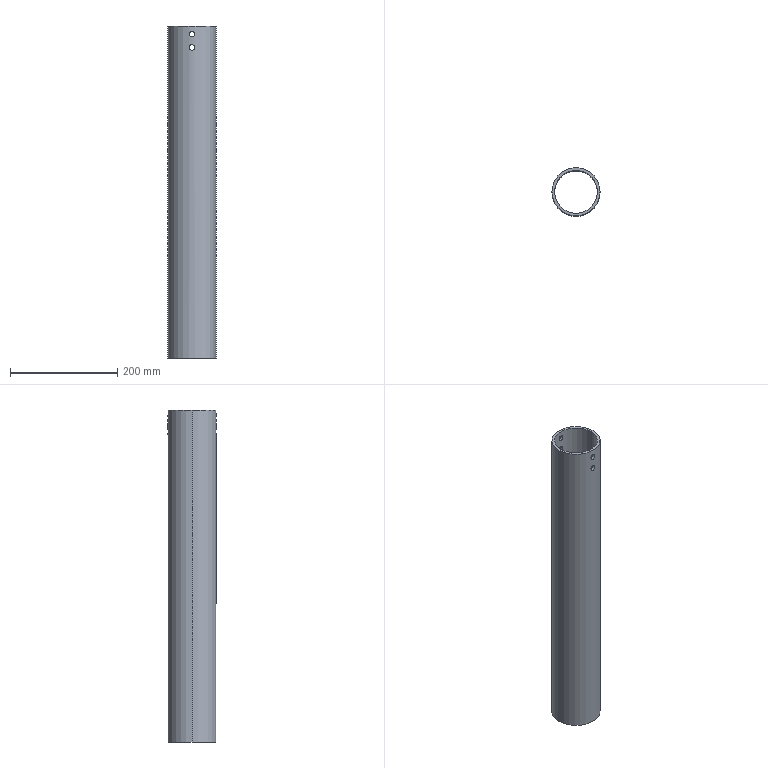Part | SolidWorks | features ICE 3, Cut 1, Extrusion 1 | 1 solid | 14 faces | box 90 x 90 x 620 mm | volume 826172 mm3 | cylinder 12 | plane 2 | commonest cylinder face diameters 10.2 x8 80 x2 90 x2
STEP:
#1=CARTESIAN_POINT('',(0.,-45.,599.9));
#2=VERTEX_POINT('',#1);
#3=CARTESIAN_POINT('',(0.,-45.,610.1));
#4=VERTEX_POINT('',#3);
#5=CARTESIAN_POINT('',(0.,-45.,599.9));
#6=CARTESIAN_POINT('',(-0.3329,-45.,599.9));
#7=CARTESIAN_POINT('',(-0.664,-44.996,599.932));
#8=CARTESIAN_POINT('',(-1.322,-44.982,600.063));
#9=CARTESIAN_POINT('',(-1.644,-44.971,600.161));
#10=CARTESIAN_POINT('',(-2.258,-44.944,600.415));
#11=CARTESIAN_POINT('',(-2.555,-44.928,600.573));
#12=CARTESIAN_POINT('',(-3.112,-44.893,600.946));
#13=CARTESIAN_POINT('',(-3.369,-44.874,601.156));
#14=CARTESIAN_POINT('',(-3.839,-44.837,601.626));
#15=CARTESIAN_POINT('',(-4.054,-44.817,601.888));
#16=CARTESIAN_POINT('',(-4.425,-44.782,602.442));
#17=CARTESIAN_POINT('',(-4.581,-44.766,602.735));
#18=CARTESIAN_POINT('',(-4.774,-44.746,603.198));
#19=CARTESIAN_POINT('',(-4.831,-44.74,603.357));
#20=CARTESIAN_POINT('',(-4.928,-44.729,603.677));
#21=CARTESIAN_POINT('',(-4.969,-44.725,603.839));
#22=CARTESIAN_POINT('',(-5.066,-44.714,604.328));
#23=CARTESIAN_POINT('',(-5.1,-44.71,604.659));
#24=CARTESIAN_POINT('',(-5.1,-44.71,605.333));
#25=CARTESIAN_POINT('',(-5.067,-44.714,605.665));
#26=CARTESIAN_POINT('',(-4.97,-44.725,606.154));
#27=CARTESIAN_POINT('',(-4.93,-44.729,606.316));
#28=CARTESIAN_POINT('',(-4.833,-44.74,606.636));
#29=CARTESIAN_POINT('',(-4.776,-44.746,606.796));
#30=CARTESIAN_POINT('',(-4.585,-44.766,607.259));
#31=CARTESIAN_POINT('',(-4.428,-44.782,607.552));
#32=CARTESIAN_POINT('',(-4.059,-44.817,608.106));
#33=CARTESIAN_POINT('',(-3.844,-44.836,608.369));
#34=CARTESIAN_POINT('',(-3.374,-44.874,608.839));
#35=CARTESIAN_POINT('',(-3.118,-44.893,609.05));
#36=CARTESIAN_POINT('',(-2.561,-44.928,609.423));
#37=CARTESIAN_POINT('',(-2.264,-44.944,609.582));
#38=CARTESIAN_POINT('',(-1.651,-44.971,609.837));
#39=CARTESIAN_POINT('',(-1.33,-44.982,609.935));
#40=CARTESIAN_POINT('',(-0.6706,-44.996,610.067));
#41=CARTESIAN_POINT('',(-0.3372,-45.,610.1));
#42=CARTESIAN_POINT('',(0.,-45.,610.1));
#43=B_SPLINE_CURVE_WITH_KNOTS('',3,(#5,#6,#7,#8,#9,#10,#11,#12,#13,#14,#15,#16,#17,#18,#19,#20,#21,#22,#23,#24,#25,#26,#27,#28,#29,#30,#31,#32,#33,#34,#35,#36,#37,#38,#39,#40,#41,#42),.UNSPECIFIED.,.F.,.F.,(4,2,2,2,2,2,2,2,2,2,2,2,2,2,2,2,2,2,4),(0.01596,0.01695,0.01795,0.01895,0.01995,0.02094,0.02194,0.02244,0.02294,0.02393,0.02493,0.02543,0.02593,0.02693,0.02792,0.02892,0.02992,0.03091,0.03191),.UNSPECIFIED.);
#44=EDGE_CURVE('',#2,#4,#43,.T.);
#45=ORIENTED_EDGE('',*,*,#44,.F.);
#46=CARTESIAN_POINT('',(0.,-40.,599.9));
#47=VERTEX_POINT('',#46);
#48=CARTESIAN_POINT('',(0.,-91.,599.9));
#49=DIRECTION('',(0.,1.,0.));
#50=VECTOR('',#49,1000.);
#51=LINE('',#48,#50);
#52=EDGE_CURVE('',#2,#47,#51,.T.);
#53=ORIENTED_EDGE('',*,*,#52,.T.);
#54=CARTESIAN_POINT('',(0.,-40.,610.1));
#55=VERTEX_POINT('',#54);
#56=CARTESIAN_POINT('',(0.,-40.,599.9));
#57=CARTESIAN_POINT('',(-0.3329,-40.,599.9));
#58=CARTESIAN_POINT('',(-0.6641,-39.996,599.932));
#59=CARTESIAN_POINT('',(-1.323,-39.979,600.063));
#60=CARTESIAN_POINT('',(-1.644,-39.967,600.161));
#61=CARTESIAN_POINT('',(-2.258,-39.937,600.415));
#62=CARTESIAN_POINT('',(-2.555,-39.919,600.573));
#63=CARTESIAN_POINT('',(-3.112,-39.88,600.946));
#64=CARTESIAN_POINT('',(-3.369,-39.859,601.156));
#65=CARTESIAN_POINT('',(-3.839,-39.816,601.626));
#66=CARTESIAN_POINT('',(-4.054,-39.794,601.888));
#67=CARTESIAN_POINT('',(-4.425,-39.755,602.442));
#68=CARTESIAN_POINT('',(-4.581,-39.737,602.734));
#69=CARTESIAN_POINT('',(-4.774,-39.714,603.197));
#70=CARTESIAN_POINT('',(-4.831,-39.707,603.357));
#71=CARTESIAN_POINT('',(-4.928,-39.695,603.677));
#72=CARTESIAN_POINT('',(-4.969,-39.69,603.839));
#73=CARTESIAN_POINT('',(-5.066,-39.678,604.328));
#74=CARTESIAN_POINT('',(-5.1,-39.674,604.659));
#75=CARTESIAN_POINT('',(-5.1,-39.674,605.334));
#76=CARTESIAN_POINT('',(-5.067,-39.678,605.665));
#77=CARTESIAN_POINT('',(-4.97,-39.69,606.154));
#78=CARTESIAN_POINT('',(-4.93,-39.695,606.316));
#79=CARTESIAN_POINT('',(-4.833,-39.707,606.637));
#80=CARTESIAN_POINT('',(-4.776,-39.714,606.796));
#81=CARTESIAN_POINT('',(-4.585,-39.737,607.259));
#82=CARTESIAN_POINT('',(-4.428,-39.755,607.552));
#83=CARTESIAN_POINT('',(-4.058,-39.794,608.107));
#84=CARTESIAN_POINT('',(-3.843,-39.816,608.369));
#85=CARTESIAN_POINT('',(-3.374,-39.858,608.839));
#86=CARTESIAN_POINT('',(-3.118,-39.879,609.05));
#87=CARTESIAN_POINT('',(-2.56,-39.919,609.423));
#88=CARTESIAN_POINT('',(-2.264,-39.937,609.582));
#89=CARTESIAN_POINT('',(-1.651,-39.967,609.837));
#90=CARTESIAN_POINT('',(-1.33,-39.979,609.935));
#91=CARTESIAN_POINT('',(-0.6707,-39.996,610.067));
#92=CARTESIAN_POINT('',(-0.3373,-40.,610.1));
#93=CARTESIAN_POINT('',(0.,-40.,610.1));
#94=B_SPLINE_CURVE_WITH_KNOTS('',3,(#56,#57,#58,#59,#60,#61,#62,#63,#64,#65,#66,#67,#68,#69,#70,#71,#72,#73,#74,#75,#76,#77,#78,#79,#80,#81,#82,#83,#84,#85,#86,#87,#88,#89,#90,#91,#92,#93),.UNSPECIFIED.,.F.,.F.,(4,2,2,2,2,2,2,2,2,2,2,2,2,2,2,2,2,2,4),(0.01596,0.01696,0.01796,0.01895,0.01995,0.02095,0.02195,0.02244,0.02294,0.02394,0.02494,0.02544,0.02593,0.02693,0.02793,0.02893,0.02992,0.03092,0.03192),.UNSPECIFIED.);
#95=EDGE_CURVE('',#47,#55,#94,.T.);
#96=ORIENTED_EDGE('',*,*,#95,.T.);
#97=CARTESIAN_POINT('',(0.,-91.,610.1));
#98=DIRECTION('',(0.,1.,0.));
#99=VECTOR('',#98,1000.);
#100=LINE('',#97,#99);
#101=EDGE_CURVE('',#4,#55,#100,.T.);
#102=ORIENTED_EDGE('',*,*,#101,.F.);
#103=EDGE_LOOP('',(#45,#53,#96,#102));
#104=FACE_OUTER_BOUND('',#103,.T.);
#105=CARTESIAN_POINT('',(0.,-91.,605.));
#106=DIRECTION('',(0.,1.,0.));
#107=DIRECTION('',(0.,0.,1.));
#108=AXIS2_PLACEMENT_3D('',#105,#106,#107);
#109=CYLINDRICAL_SURFACE('',#108,5.1);
#110=ADVANCED_FACE('',(#104),#109,.F.);
#111=CARTESIAN_POINT('',(0.,40.,610.1));
#112=VERTEX_POINT('',#111);
#113=CARTESIAN_POINT('',(0.,40.,599.9));
#114=VERTEX_POINT('',#113);
#115=CARTESIAN_POINT('',(0.,40.,610.1));
#116=CARTESIAN_POINT('',(-0.3373,40.,610.1));
#117=CARTESIAN_POINT('',(-0.669,39.996,610.067));
#118=CARTESIAN_POINT('',(-1.158,39.984,609.97));
#119=CARTESIAN_POINT('',(-1.32,39.979,609.929));
#120=CARTESIAN_POINT('',(-1.641,39.967,609.832));
#121=CARTESIAN_POINT('',(-1.8,39.96,609.775));
#122=CARTESIAN_POINT('',(-2.263,39.937,609.583));
#123=CARTESIAN_POINT('',(-2.556,39.919,609.426));
#124=CARTESIAN_POINT('',(-3.11,39.88,609.056));
#125=CARTESIAN_POINT('',(-3.372,39.858,608.841));
#126=CARTESIAN_POINT('',(-3.842,39.816,608.37));
#127=CARTESIAN_POINT('',(-4.053,39.795,608.114));
#128=CARTESIAN_POINT('',(-4.426,39.755,607.556));
#129=CARTESIAN_POINT('',(-4.584,39.737,607.26));
#130=CARTESIAN_POINT('',(-4.838,39.707,606.646));
#131=CARTESIAN_POINT('',(-4.936,39.694,606.325));
#132=CARTESIAN_POINT('',(-5.067,39.678,605.666));
#133=CARTESIAN_POINT('',(-5.1,39.674,605.335));
#134=CARTESIAN_POINT('',(-5.1,39.674,604.669));
#135=CARTESIAN_POINT('',(-5.067,39.678,604.331));
#136=CARTESIAN_POINT('',(-4.936,39.694,603.676));
#137=CARTESIAN_POINT('',(-4.84,39.706,603.358));
#138=CARTESIAN_POINT('',(-4.648,39.729,602.895));
#139=CARTESIAN_POINT('',(-4.576,39.737,602.742));
#140=CARTESIAN_POINT('',(-4.418,39.755,602.447));
#141=CARTESIAN_POINT('',(-4.332,39.765,602.304));
#142=CARTESIAN_POINT('',(-4.055,39.794,601.89));
#143=CARTESIAN_POINT('',(-3.844,39.816,601.632));
#144=CARTESIAN_POINT('',(-3.369,39.859,601.156));
#145=CARTESIAN_POINT('',(-3.111,39.88,600.945));
#146=CARTESIAN_POINT('',(-2.697,39.909,600.669));
#147=CARTESIAN_POINT('',(-2.555,39.919,600.583));
#148=CARTESIAN_POINT('',(-2.259,39.936,600.425));
#149=CARTESIAN_POINT('',(-2.107,39.945,600.352));
#150=CARTESIAN_POINT('',(-1.644,39.967,600.161));
#151=CARTESIAN_POINT('',(-1.326,39.979,600.064));
#152=CARTESIAN_POINT('',(-0.6713,39.996,599.933));
#153=CARTESIAN_POINT('',(-0.333,40.,599.9));
#154=CARTESIAN_POINT('',(0.,40.,599.9));
#155=B_SPLINE_CURVE_WITH_KNOTS('',3,(#115,#116,#117,#118,#119,#120,#121,#122,#123,#124,#125,#126,#127,#128,#129,#130,#131,#132,#133,#134,#135,#136,#137,#138,#139,#140,#141,#142,#143,#144,#145,#146,#147,#148,#149,#150,#151,#152,#153,#154),.UNSPECIFIED.,.F.,.F.,(4,2,2,2,2,2,2,2,2,2,2,2,2,2,2,2,2,2,2,4),(0.,0.0009976,0.001496,0.001995,0.002993,0.00399,0.004988,0.005985,0.006983,0.007981,0.008978,0.009976,0.01047,0.01097,0.01197,0.01297,0.01347,0.01397,0.01496,0.01596),.UNSPECIFIED.);
#156=EDGE_CURVE('',#112,#114,#155,.T.);
#157=ORIENTED_EDGE('',*,*,#156,.T.);
#158=CARTESIAN_POINT('',(0.,45.,599.9));
#159=VERTEX_POINT('',#158);
#160=CARTESIAN_POINT('',(0.,-91.,599.9));
#161=DIRECTION('',(0.,1.,0.));
#162=VECTOR('',#161,1000.);
#163=LINE('',#160,#162);
#164=EDGE_CURVE('',#114,#159,#163,.T.);
#165=ORIENTED_EDGE('',*,*,#164,.T.);
#166=CARTESIAN_POINT('',(0.,45.,610.1));
#167=VERTEX_POINT('',#166);
#168=CARTESIAN_POINT('',(0.,45.,610.1));
#169=CARTESIAN_POINT('',(-0.3373,45.,610.1));
#170=CARTESIAN_POINT('',(-0.6688,44.996,610.067));
#171=CARTESIAN_POINT('',(-1.158,44.985,609.97));
#172=CARTESIAN_POINT('',(-1.32,44.981,609.929));
#173=CARTESIAN_POINT('',(-1.64,44.97,609.832));
#174=CARTESIAN_POINT('',(-1.8,44.964,609.775));
#175=CARTESIAN_POINT('',(-2.263,44.944,609.583));
#176=CARTESIAN_POINT('',(-2.556,44.928,609.426));
#177=CARTESIAN_POINT('',(-3.11,44.893,609.056));
#178=CARTESIAN_POINT('',(-3.372,44.874,608.841));
#179=CARTESIAN_POINT('',(-3.842,44.836,608.37));
#180=CARTESIAN_POINT('',(-4.053,44.818,608.114));
#181=CARTESIAN_POINT('',(-4.426,44.782,607.556));
#182=CARTESIAN_POINT('',(-4.584,44.766,607.26));
#183=CARTESIAN_POINT('',(-4.838,44.739,606.646));
#184=CARTESIAN_POINT('',(-4.936,44.728,606.324));
#185=CARTESIAN_POINT('',(-5.067,44.714,605.666));
#186=CARTESIAN_POINT('',(-5.1,44.71,605.335));
#187=CARTESIAN_POINT('',(-5.1,44.71,604.669));
#188=CARTESIAN_POINT('',(-5.067,44.714,604.331));
#189=CARTESIAN_POINT('',(-4.937,44.728,603.676));
#190=CARTESIAN_POINT('',(-4.84,44.739,603.358));
#191=CARTESIAN_POINT('',(-4.648,44.759,602.895));
#192=CARTESIAN_POINT('',(-4.576,44.767,602.742));
#193=CARTESIAN_POINT('',(-4.418,44.783,602.447));
#194=CARTESIAN_POINT('',(-4.332,44.791,602.304));
#195=CARTESIAN_POINT('',(-4.056,44.817,601.89));
#196=CARTESIAN_POINT('',(-3.845,44.836,601.632));
#197=CARTESIAN_POINT('',(-3.369,44.874,601.156));
#198=CARTESIAN_POINT('',(-3.111,44.893,600.945));
#199=CARTESIAN_POINT('',(-2.697,44.919,600.668));
#200=CARTESIAN_POINT('',(-2.554,44.928,600.583));
#201=CARTESIAN_POINT('',(-2.259,44.943,600.425));
#202=CARTESIAN_POINT('',(-2.106,44.951,600.352));
#203=CARTESIAN_POINT('',(-1.643,44.971,600.16));
#204=CARTESIAN_POINT('',(-1.325,44.982,600.064));
#205=CARTESIAN_POINT('',(-0.6712,44.996,599.933));
#206=CARTESIAN_POINT('',(-0.333,45.,599.9));
#207=CARTESIAN_POINT('',(0.,45.,599.9));
#208=B_SPLINE_CURVE_WITH_KNOTS('',3,(#168,#169,#170,#171,#172,#173,#174,#175,#176,#177,#178,#179,#180,#181,#182,#183,#184,#185,#186,#187,#188,#189,#190,#191,#192,#193,#194,#195,#196,#197,#198,#199,#200,#201,#202,#203,#204,#205,#206,#207),.UNSPECIFIED.,.F.,.F.,(4,2,2,2,2,2,2,2,2,2,2,2,2,2,2,2,2,2,2,4),(0.,0.0009974,0.001496,0.001995,0.002992,0.003989,0.004987,0.005984,0.006982,0.007979,0.008976,0.009974,0.01047,0.01097,0.01197,0.01297,0.01346,0.01396,0.01496,0.01596),.UNSPECIFIED.);
#209=EDGE_CURVE('',#167,#159,#208,.T.);
#210=ORIENTED_EDGE('',*,*,#209,.F.);
#211=CARTESIAN_POINT('',(0.,-91.,610.1));
#212=DIRECTION('',(0.,1.,0.));
#213=VECTOR('',#212,1000.);
#214=LINE('',#211,#213);
#215=EDGE_CURVE('',#112,#167,#214,.T.);
#216=ORIENTED_EDGE('',*,*,#215,.F.);
#217=EDGE_LOOP('',(#157,#165,#210,#216));
#218=FACE_OUTER_BOUND('',#217,.T.);
#219=CARTESIAN_POINT('',(0.,-91.,605.));
#220=DIRECTION('',(0.,1.,0.));
#221=DIRECTION('',(0.,0.,1.));
#222=AXIS2_PLACEMENT_3D('',#219,#220,#221);
#223=CYLINDRICAL_SURFACE('',#222,5.1);
#224=ADVANCED_FACE('',(#218),#223,.F.);
#225=CARTESIAN_POINT('',(0.,-45.,574.9));
#226=VERTEX_POINT('',#225);
#227=CARTESIAN_POINT('',(0.,-45.,585.1));
#228=VERTEX_POINT('',#227);
#229=CARTESIAN_POINT('',(0.,-45.,574.9));
#230=CARTESIAN_POINT('',(-0.3329,-45.,574.9));
#231=CARTESIAN_POINT('',(-0.664,-44.996,574.932));
#232=CARTESIAN_POINT('',(-1.322,-44.982,575.063));
#233=CARTESIAN_POINT('',(-1.644,-44.971,575.161));
#234=CARTESIAN_POINT('',(-2.258,-44.944,575.415));
#235=CARTESIAN_POINT('',(-2.555,-44.928,575.573));
#236=CARTESIAN_POINT('',(-3.112,-44.893,575.946));
#237=CARTESIAN_POINT('',(-3.369,-44.874,576.156));
#238=CARTESIAN_POINT('',(-3.839,-44.837,576.626));
#239=CARTESIAN_POINT('',(-4.054,-44.817,576.888));
#240=CARTESIAN_POINT('',(-4.425,-44.782,577.442));
#241=CARTESIAN_POINT('',(-4.581,-44.766,577.735));
#242=CARTESIAN_POINT('',(-4.774,-44.746,578.198));
#243=CARTESIAN_POINT('',(-4.831,-44.74,578.357));
#244=CARTESIAN_POINT('',(-4.928,-44.729,578.677));
#245=CARTESIAN_POINT('',(-4.969,-44.725,578.839));
#246=CARTESIAN_POINT('',(-5.066,-44.714,579.328));
#247=CARTESIAN_POINT('',(-5.1,-44.71,579.659));
#248=CARTESIAN_POINT('',(-5.1,-44.71,580.333));
#249=CARTESIAN_POINT('',(-5.067,-44.714,580.665));
#250=CARTESIAN_POINT('',(-4.97,-44.725,581.154));
#251=CARTESIAN_POINT('',(-4.93,-44.729,581.316));
#252=CARTESIAN_POINT('',(-4.833,-44.74,581.636));
#253=CARTESIAN_POINT('',(-4.776,-44.746,581.796));
#254=CARTESIAN_POINT('',(-4.585,-44.766,582.259));
#255=CARTESIAN_POINT('',(-4.428,-44.782,582.552));
#256=CARTESIAN_POINT('',(-4.059,-44.817,583.106));
#257=CARTESIAN_POINT('',(-3.844,-44.836,583.369));
#258=CARTESIAN_POINT('',(-3.374,-44.874,583.839));
#259=CARTESIAN_POINT('',(-3.118,-44.893,584.05));
#260=CARTESIAN_POINT('',(-2.561,-44.928,584.423));
#261=CARTESIAN_POINT('',(-2.264,-44.944,584.582));
#262=CARTESIAN_POINT('',(-1.651,-44.971,584.837));
#263=CARTESIAN_POINT('',(-1.33,-44.982,584.935));
#264=CARTESIAN_POINT('',(-0.6706,-44.996,585.067));
#265=CARTESIAN_POINT('',(-0.3372,-45.,585.1));
#266=CARTESIAN_POINT('',(0.,-45.,585.1));
#267=B_SPLINE_CURVE_WITH_KNOTS('',3,(#229,#230,#231,#232,#233,#234,#235,#236,#237,#238,#239,#240,#241,#242,#243,#244,#245,#246,#247,#248,#249,#250,#251,#252,#253,#254,#255,#256,#257,#258,#259,#260,#261,#262,#263,#264,#265,#266),.UNSPECIFIED.,.F.,.F.,(4,2,2,2,2,2,2,2,2,2,2,2,2,2,2,2,2,2,4),(0.01596,0.01695,0.01795,0.01895,0.01995,0.02094,0.02194,0.02244,0.02294,0.02393,0.02493,0.02543,0.02593,0.02693,0.02792,0.02892,0.02992,0.03091,0.03191),.UNSPECIFIED.);
#268=EDGE_CURVE('',#226,#228,#267,.T.);
#269=ORIENTED_EDGE('',*,*,#268,.F.);
#270=CARTESIAN_POINT('',(0.,-40.,574.9));
#271=VERTEX_POINT('',#270);
#272=CARTESIAN_POINT('',(0.,-91.,574.9));
#273=DIRECTION('',(0.,1.,0.));
#274=VECTOR('',#273,1000.);
#275=LINE('',#272,#274);
#276=EDGE_CURVE('',#226,#271,#275,.T.);
#277=ORIENTED_EDGE('',*,*,#276,.T.);
#278=CARTESIAN_POINT('',(0.,-40.,585.1));
#279=VERTEX_POINT('',#278);
#280=CARTESIAN_POINT('',(0.,-40.,574.9));
#281=CARTESIAN_POINT('',(-0.3329,-40.,574.9));
#282=CARTESIAN_POINT('',(-0.6641,-39.996,574.932));
#283=CARTESIAN_POINT('',(-1.323,-39.979,575.063));
#284=CARTESIAN_POINT('',(-1.644,-39.967,575.161));
#285=CARTESIAN_POINT('',(-2.258,-39.937,575.415));
#286=CARTESIAN_POINT('',(-2.555,-39.919,575.573));
#287=CARTESIAN_POINT('',(-3.112,-39.88,575.946));
#288=CARTESIAN_POINT('',(-3.369,-39.859,576.156));
#289=CARTESIAN_POINT('',(-3.839,-39.816,576.626));
#290=CARTESIAN_POINT('',(-4.054,-39.794,576.888));
#291=CARTESIAN_POINT('',(-4.425,-39.755,577.442));
#292=CARTESIAN_POINT('',(-4.581,-39.737,577.734));
#293=CARTESIAN_POINT('',(-4.774,-39.714,578.197));
#294=CARTESIAN_POINT('',(-4.831,-39.707,578.357));
#295=CARTESIAN_POINT('',(-4.928,-39.695,578.677));
#296=CARTESIAN_POINT('',(-4.969,-39.69,578.839));
#297=CARTESIAN_POINT('',(-5.066,-39.678,579.328));
#298=CARTESIAN_POINT('',(-5.1,-39.674,579.659));
#299=CARTESIAN_POINT('',(-5.1,-39.674,580.334));
#300=CARTESIAN_POINT('',(-5.067,-39.678,580.665));
#301=CARTESIAN_POINT('',(-4.97,-39.69,581.154));
#302=CARTESIAN_POINT('',(-4.93,-39.695,581.316));
#303=CARTESIAN_POINT('',(-4.833,-39.707,581.637));
#304=CARTESIAN_POINT('',(-4.776,-39.714,581.796));
#305=CARTESIAN_POINT('',(-4.585,-39.737,582.259));
#306=CARTESIAN_POINT('',(-4.428,-39.755,582.552));
#307=CARTESIAN_POINT('',(-4.058,-39.794,583.107));
#308=CARTESIAN_POINT('',(-3.843,-39.816,583.369));
#309=CARTESIAN_POINT('',(-3.374,-39.858,583.839));
#310=CARTESIAN_POINT('',(-3.118,-39.879,584.05));
#311=CARTESIAN_POINT('',(-2.56,-39.919,584.423));
#312=CARTESIAN_POINT('',(-2.264,-39.937,584.582));
#313=CARTESIAN_POINT('',(-1.651,-39.967,584.837));
#314=CARTESIAN_POINT('',(-1.33,-39.979,584.935));
#315=CARTESIAN_POINT('',(-0.6707,-39.996,585.067));
#316=CARTESIAN_POINT('',(-0.3373,-40.,585.1));
#317=CARTESIAN_POINT('',(0.,-40.,585.1));
#318=B_SPLINE_CURVE_WITH_KNOTS('',3,(#280,#281,#282,#283,#284,#285,#286,#287,#288,#289,#290,#291,#292,#293,#294,#295,#296,#297,#298,#299,#300,#301,#302,#303,#304,#305,#306,#307,#308,#309,#310,#311,#312,#313,#314,#315,#316,#317),.UNSPECIFIED.,.F.,.F.,(4,2,2,2,2,2,2,2,2,2,2,2,2,2,2,2,2,2,4),(0.01596,0.01696,0.01796,0.01895,0.01995,0.02095,0.02195,0.02244,0.02294,0.02394,0.02494,0.02544,0.02593,0.02693,0.02793,0.02893,0.02992,0.03092,0.03192),.UNSPECIFIED.);
#319=EDGE_CURVE('',#271,#279,#318,.T.);
#320=ORIENTED_EDGE('',*,*,#319,.T.);
#321=CARTESIAN_POINT('',(0.,-91.,585.1));
#322=DIRECTION('',(0.,1.,0.));
#323=VECTOR('',#322,1000.);
#324=LINE('',#321,#323);
#325=EDGE_CURVE('',#228,#279,#324,.T.);
#326=ORIENTED_EDGE('',*,*,#325,.F.);
#327=EDGE_LOOP('',(#269,#277,#320,#326));
#328=FACE_OUTER_BOUND('',#327,.T.);
#329=CARTESIAN_POINT('',(0.,-91.,580.));
#330=DIRECTION('',(0.,1.,0.));
#331=DIRECTION('',(0.,0.,1.));
#332=AXIS2_PLACEMENT_3D('',#329,#330,#331);
#333=CYLINDRICAL_SURFACE('',#332,5.1);
#334=ADVANCED_FACE('',(#328),#333,.F.);
#335=CARTESIAN_POINT('',(0.,40.,585.1));
#336=VERTEX_POINT('',#335);
#337=CARTESIAN_POINT('',(0.,40.,574.9));
#338=VERTEX_POINT('',#337);
#339=CARTESIAN_POINT('',(0.,40.,585.1));
#340=CARTESIAN_POINT('',(-0.3373,40.,585.1));
#341=CARTESIAN_POINT('',(-0.669,39.996,585.067));
#342=CARTESIAN_POINT('',(-1.158,39.984,584.97));
#343=CARTESIAN_POINT('',(-1.32,39.979,584.929));
#344=CARTESIAN_POINT('',(-1.641,39.967,584.832));
#345=CARTESIAN_POINT('',(-1.8,39.96,584.775));
#346=CARTESIAN_POINT('',(-2.263,39.937,584.583));
#347=CARTESIAN_POINT('',(-2.556,39.919,584.426));
#348=CARTESIAN_POINT('',(-3.11,39.88,584.056));
#349=CARTESIAN_POINT('',(-3.372,39.858,583.841));
#350=CARTESIAN_POINT('',(-3.842,39.816,583.37));
#351=CARTESIAN_POINT('',(-4.053,39.795,583.114));
#352=CARTESIAN_POINT('',(-4.426,39.755,582.556));
#353=CARTESIAN_POINT('',(-4.584,39.737,582.26));
#354=CARTESIAN_POINT('',(-4.838,39.707,581.646));
#355=CARTESIAN_POINT('',(-4.936,39.694,581.325));
#356=CARTESIAN_POINT('',(-5.067,39.678,580.666));
#357=CARTESIAN_POINT('',(-5.1,39.674,580.335));
#358=CARTESIAN_POINT('',(-5.1,39.674,579.669));
#359=CARTESIAN_POINT('',(-5.067,39.678,579.331));
#360=CARTESIAN_POINT('',(-4.936,39.694,578.676));
#361=CARTESIAN_POINT('',(-4.84,39.706,578.358));
#362=CARTESIAN_POINT('',(-4.648,39.729,577.895));
#363=CARTESIAN_POINT('',(-4.576,39.737,577.742));
#364=CARTESIAN_POINT('',(-4.418,39.755,577.447));
#365=CARTESIAN_POINT('',(-4.332,39.765,577.304));
#366=CARTESIAN_POINT('',(-4.055,39.794,576.89));
#367=CARTESIAN_POINT('',(-3.844,39.816,576.632));
#368=CARTESIAN_POINT('',(-3.369,39.859,576.156));
#369=CARTESIAN_POINT('',(-3.111,39.88,575.945));
#370=CARTESIAN_POINT('',(-2.697,39.909,575.669));
#371=CARTESIAN_POINT('',(-2.555,39.919,575.583));
#372=CARTESIAN_POINT('',(-2.259,39.936,575.425));
#373=CARTESIAN_POINT('',(-2.107,39.945,575.352));
#374=CARTESIAN_POINT('',(-1.644,39.967,575.161));
#375=CARTESIAN_POINT('',(-1.326,39.979,575.064));
#376=CARTESIAN_POINT('',(-0.6713,39.996,574.933));
#377=CARTESIAN_POINT('',(-0.333,40.,574.9));
#378=CARTESIAN_POINT('',(0.,40.,574.9));
#379=B_SPLINE_CURVE_WITH_KNOTS('',3,(#339,#340,#341,#342,#343,#344,#345,#346,#347,#348,#349,#350,#351,#352,#353,#354,#355,#356,#357,#358,#359,#360,#361,#362,#363,#364,#365,#366,#367,#368,#369,#370,#371,#372,#373,#374,#375,#376,#377,#378),.UNSPECIFIED.,.F.,.F.,(4,2,2,2,2,2,2,2,2,2,2,2,2,2,2,2,2,2,2,4),(0.,0.0009976,0.001496,0.001995,0.002993,0.00399,0.004988,0.005985,0.006983,0.007981,0.008978,0.009976,0.01047,0.01097,0.01197,0.01297,0.01347,0.01397,0.01496,0.01596),.UNSPECIFIED.);
#380=EDGE_CURVE('',#336,#338,#379,.T.);
#381=ORIENTED_EDGE('',*,*,#380,.T.);
#382=CARTESIAN_POINT('',(0.,45.,574.9));
#383=VERTEX_POINT('',#382);
#384=CARTESIAN_POINT('',(0.,-91.,574.9));
#385=DIRECTION('',(0.,1.,0.));
#386=VECTOR('',#385,1000.);
#387=LINE('',#384,#386);
#388=EDGE_CURVE('',#338,#383,#387,.T.);
#389=ORIENTED_EDGE('',*,*,#388,.T.);
#390=CARTESIAN_POINT('',(0.,45.,585.1));
#391=VERTEX_POINT('',#390);
#392=CARTESIAN_POINT('',(0.,45.,585.1));
#393=CARTESIAN_POINT('',(-0.3373,45.,585.1));
#394=CARTESIAN_POINT('',(-0.6688,44.996,585.067));
#395=CARTESIAN_POINT('',(-1.158,44.985,584.97));
#396=CARTESIAN_POINT('',(-1.32,44.981,584.929));
#397=CARTESIAN_POINT('',(-1.64,44.97,584.832));
#398=CARTESIAN_POINT('',(-1.8,44.964,584.775));
#399=CARTESIAN_POINT('',(-2.263,44.944,584.583));
#400=CARTESIAN_POINT('',(-2.556,44.928,584.426));
#401=CARTESIAN_POINT('',(-3.11,44.893,584.056));
#402=CARTESIAN_POINT('',(-3.372,44.874,583.841));
#403=CARTESIAN_POINT('',(-3.842,44.836,583.37));
#404=CARTESIAN_POINT('',(-4.053,44.818,583.114));
#405=CARTESIAN_POINT('',(-4.426,44.782,582.556));
#406=CARTESIAN_POINT('',(-4.584,44.766,582.26));
#407=CARTESIAN_POINT('',(-4.838,44.739,581.646));
#408=CARTESIAN_POINT('',(-4.936,44.728,581.324));
#409=CARTESIAN_POINT('',(-5.067,44.714,580.666));
#410=CARTESIAN_POINT('',(-5.1,44.71,580.335));
#411=CARTESIAN_POINT('',(-5.1,44.71,579.669));
#412=CARTESIAN_POINT('',(-5.067,44.714,579.331));
#413=CARTESIAN_POINT('',(-4.937,44.728,578.676));
#414=CARTESIAN_POINT('',(-4.84,44.739,578.358));
#415=CARTESIAN_POINT('',(-4.648,44.759,577.895));
#416=CARTESIAN_POINT('',(-4.576,44.767,577.742));
#417=CARTESIAN_POINT('',(-4.418,44.783,577.447));
#418=CARTESIAN_POINT('',(-4.332,44.791,577.304));
#419=CARTESIAN_POINT('',(-4.056,44.817,576.89));
#420=CARTESIAN_POINT('',(-3.845,44.836,576.632));
#421=CARTESIAN_POINT('',(-3.369,44.874,576.156));
#422=CARTESIAN_POINT('',(-3.111,44.893,575.945));
#423=CARTESIAN_POINT('',(-2.697,44.919,575.668));
#424=CARTESIAN_POINT('',(-2.554,44.928,575.583));
#425=CARTESIAN_POINT('',(-2.259,44.943,575.425));
#426=CARTESIAN_POINT('',(-2.106,44.951,575.352));
#427=CARTESIAN_POINT('',(-1.643,44.971,575.16));
#428=CARTESIAN_POINT('',(-1.325,44.982,575.064));
#429=CARTESIAN_POINT('',(-0.6712,44.996,574.933));
#430=CARTESIAN_POINT('',(-0.333,45.,574.9));
#431=CARTESIAN_POINT('',(0.,45.,574.9));
#432=B_SPLINE_CURVE_WITH_KNOTS('',3,(#392,#393,#394,#395,#396,#397,#398,#399,#400,#401,#402,#403,#404,#405,#406,#407,#408,#409,#410,#411,#412,#413,#414,#415,#416,#417,#418,#419,#420,#421,#422,#423,#424,#425,#426,#427,#428,#429,#430,#431),.UNSPECIFIED.,.F.,.F.,(4,2,2,2,2,2,2,2,2,2,2,2,2,2,2,2,2,2,2,4),(0.,0.0009974,0.001496,0.001995,0.002992,0.003989,0.004987,0.005984,0.006982,0.007979,0.008976,0.009974,0.01047,0.01097,0.01197,0.01297,0.01346,0.01396,0.01496,0.01596),.UNSPECIFIED.);
#433=EDGE_CURVE('',#391,#383,#432,.T.);
#434=ORIENTED_EDGE('',*,*,#433,.F.);
#435=CARTESIAN_POINT('',(0.,-91.,585.1));
#436=DIRECTION('',(0.,1.,0.));
#437=VECTOR('',#436,1000.);
#438=LINE('',#435,#437);
#439=EDGE_CURVE('',#336,#391,#438,.T.);
#440=ORIENTED_EDGE('',*,*,#439,.F.);
#441=EDGE_LOOP('',(#381,#389,#434,#440));
#442=FACE_OUTER_BOUND('',#441,.T.);
#443=CARTESIAN_POINT('',(0.,-91.,580.));
#444=DIRECTION('',(0.,1.,0.));
#445=DIRECTION('',(0.,0.,1.));
#446=AXIS2_PLACEMENT_3D('',#443,#444,#445);
#447=CYLINDRICAL_SURFACE('',#446,5.1);
#448=ADVANCED_FACE('',(#442),#447,.F.);
#449=CARTESIAN_POINT('',(0.,-40.,585.1));
#450=CARTESIAN_POINT('',(0.3373,-40.,585.1));
#451=CARTESIAN_POINT('',(0.669,-39.996,585.067));
#452=CARTESIAN_POINT('',(1.158,-39.984,584.97));
#453=CARTESIAN_POINT('',(1.32,-39.979,584.929));
#454=CARTESIAN_POINT('',(1.641,-39.967,584.832));
#455=CARTESIAN_POINT('',(1.8,-39.96,584.775));
#456=CARTESIAN_POINT('',(2.263,-39.937,584.583));
#457=CARTESIAN_POINT('',(2.556,-39.919,584.426));
#458=CARTESIAN_POINT('',(3.11,-39.88,584.056));
#459=CARTESIAN_POINT('',(3.372,-39.858,583.841));
#460=CARTESIAN_POINT('',(3.842,-39.816,583.37));
#461=CARTESIAN_POINT('',(4.053,-39.795,583.114));
#462=CARTESIAN_POINT('',(4.426,-39.755,582.556));
#463=CARTESIAN_POINT('',(4.584,-39.737,582.26));
#464=CARTESIAN_POINT('',(4.838,-39.707,581.646));
#465=CARTESIAN_POINT('',(4.936,-39.694,581.325));
#466=CARTESIAN_POINT('',(5.067,-39.678,580.666));
#467=CARTESIAN_POINT('',(5.1,-39.674,580.335));
#468=CARTESIAN_POINT('',(5.1,-39.674,579.669));
#469=CARTESIAN_POINT('',(5.067,-39.678,579.331));
#470=CARTESIAN_POINT('',(4.936,-39.694,578.676));
#471=CARTESIAN_POINT('',(4.84,-39.706,578.358));
#472=CARTESIAN_POINT('',(4.648,-39.729,577.895));
#473=CARTESIAN_POINT('',(4.576,-39.737,577.742));
#474=CARTESIAN_POINT('',(4.418,-39.755,577.447));
#475=CARTESIAN_POINT('',(4.332,-39.765,577.304));
#476=CARTESIAN_POINT('',(4.055,-39.794,576.89));
#477=CARTESIAN_POINT('',(3.844,-39.816,576.632));
#478=CARTESIAN_POINT('',(3.369,-39.859,576.156));
#479=CARTESIAN_POINT('',(3.111,-39.88,575.945));
#480=CARTESIAN_POINT('',(2.697,-39.909,575.669));
#481=CARTESIAN_POINT('',(2.555,-39.919,575.583));
#482=CARTESIAN_POINT('',(2.259,-39.936,575.425));
#483=CARTESIAN_POINT('',(2.107,-39.945,575.352));
#484=CARTESIAN_POINT('',(1.644,-39.967,575.161));
#485=CARTESIAN_POINT('',(1.326,-39.979,575.064));
#486=CARTESIAN_POINT('',(0.6713,-39.996,574.933));
#487=CARTESIAN_POINT('',(0.333,-40.,574.9));
#488=CARTESIAN_POINT('',(0.,-40.,574.9));
#489=B_SPLINE_CURVE_WITH_KNOTS('',3,(#449,#450,#451,#452,#453,#454,#455,#456,#457,#458,#459,#460,#461,#462,#463,#464,#465,#466,#467,#468,#469,#470,#471,#472,#473,#474,#475,#476,#477,#478,#479,#480,#481,#482,#483,#484,#485,#486,#487,#488),.UNSPECIFIED.,.F.,.F.,(4,2,2,2,2,2,2,2,2,2,2,2,2,2,2,2,2,2,2,4),(0.,0.0009976,0.001496,0.001995,0.002993,0.00399,0.004988,0.005985,0.006983,0.007981,0.008978,0.009976,0.01047,0.01097,0.01197,0.01297,0.01347,0.01397,0.01496,0.01596),.UNSPECIFIED.);
#490=EDGE_CURVE('',#279,#271,#489,.T.);
#491=ORIENTED_EDGE('',*,*,#490,.F.);
#492=ORIENTED_EDGE('',*,*,#319,.F.);
#493=EDGE_LOOP('',(#491,#492));
#494=FACE_BOUND('',#493,.T.);
#495=CARTESIAN_POINT('',(0.,-40.,610.1));
#496=CARTESIAN_POINT('',(0.3373,-40.,610.1));
#497=CARTESIAN_POINT('',(0.669,-39.996,610.067));
#498=CARTESIAN_POINT('',(1.158,-39.984,609.97));
#499=CARTESIAN_POINT('',(1.32,-39.979,609.929));
#500=CARTESIAN_POINT('',(1.641,-39.967,609.832));
#501=CARTESIAN_POINT('',(1.8,-39.96,609.775));
#502=CARTESIAN_POINT('',(2.263,-39.937,609.583));
#503=CARTESIAN_POINT('',(2.556,-39.919,609.426));
#504=CARTESIAN_POINT('',(3.11,-39.88,609.056));
#505=CARTESIAN_POINT('',(3.372,-39.858,608.841));
#506=CARTESIAN_POINT('',(3.842,-39.816,608.37));
#507=CARTESIAN_POINT('',(4.053,-39.795,608.114));
#508=CARTESIAN_POINT('',(4.426,-39.755,607.556));
#509=CARTESIAN_POINT('',(4.584,-39.737,607.26));
#510=CARTESIAN_POINT('',(4.838,-39.707,606.646));
#511=CARTESIAN_POINT('',(4.936,-39.694,606.325));
#512=CARTESIAN_POINT('',(5.067,-39.678,605.666));
#513=CARTESIAN_POINT('',(5.1,-39.674,605.335));
#514=CARTESIAN_POINT('',(5.1,-39.674,604.669));
#515=CARTESIAN_POINT('',(5.067,-39.678,604.331));
#516=CARTESIAN_POINT('',(4.936,-39.694,603.676));
#517=CARTESIAN_POINT('',(4.84,-39.706,603.358));
#518=CARTESIAN_POINT('',(4.648,-39.729,602.895));
#519=CARTESIAN_POINT('',(4.576,-39.737,602.742));
#520=CARTESIAN_POINT('',(4.418,-39.755,602.447));
#521=CARTESIAN_POINT('',(4.332,-39.765,602.304));
#522=CARTESIAN_POINT('',(4.055,-39.794,601.89));
#523=CARTESIAN_POINT('',(3.844,-39.816,601.632));
#524=CARTESIAN_POINT('',(3.369,-39.859,601.156));
#525=CARTESIAN_POINT('',(3.111,-39.88,600.945));
#526=CARTESIAN_POINT('',(2.697,-39.909,600.669));
#527=CARTESIAN_POINT('',(2.555,-39.919,600.583));
#528=CARTESIAN_POINT('',(2.259,-39.936,600.425));
#529=CARTESIAN_POINT('',(2.107,-39.945,600.352));
#530=CARTESIAN_POINT('',(1.644,-39.967,600.161));
#531=CARTESIAN_POINT('',(1.326,-39.979,600.064));
#532=CARTESIAN_POINT('',(0.6713,-39.996,599.933));
#533=CARTESIAN_POINT('',(0.333,-40.,599.9));
#534=CARTESIAN_POINT('',(0.,-40.,599.9));
#535=B_SPLINE_CURVE_WITH_KNOTS('',3,(#495,#496,#497,#498,#499,#500,#501,#502,#503,#504,#505,#506,#507,#508,#509,#510,#511,#512,#513,#514,#515,#516,#517,#518,#519,#520,#521,#522,#523,#524,#525,#526,#527,#528,#529,#530,#531,#532,#533,#534),.UNSPECIFIED.,.F.,.F.,(4,2,2,2,2,2,2,2,2,2,2,2,2,2,2,2,2,2,2,4),(0.,0.0009976,0.001496,0.001995,0.002993,0.00399,0.004988,0.005985,0.006983,0.007981,0.008978,0.009976,0.01047,0.01097,0.01197,0.01297,0.01347,0.01397,0.01496,0.01596),.UNSPECIFIED.);
#536=EDGE_CURVE('',#55,#47,#535,.T.);
#537=ORIENTED_EDGE('',*,*,#536,.F.);
#538=ORIENTED_EDGE('',*,*,#95,.F.);
#539=EDGE_LOOP('',(#537,#538));
#540=FACE_BOUND('',#539,.T.);
#541=CARTESIAN_POINT('',(-40.,0.,620.));
#542=VERTEX_POINT('',#541);
#543=CARTESIAN_POINT('',(40.,0.,620.));
#544=VERTEX_POINT('',#543);
#545=CARTESIAN_POINT('',(0.,0.,620.));
#546=DIRECTION('',(0.,0.,1.));
#547=DIRECTION('',(1.,0.,0.));
#548=AXIS2_PLACEMENT_3D('',#545,#546,#547);
#549=CIRCLE('',#548,40.);
#550=EDGE_CURVE('',#542,#544,#549,.T.);
#551=ORIENTED_EDGE('',*,*,#550,.T.);
#552=CARTESIAN_POINT('',(40.,0.,0.));
#553=VERTEX_POINT('',#552);
#554=CARTESIAN_POINT('',(40.,0.,40.));
#555=DIRECTION('',(0.,0.,-1.));
#556=VECTOR('',#555,1000.);
#557=LINE('',#554,#556);
#558=EDGE_CURVE('',#544,#553,#557,.T.);
#559=ORIENTED_EDGE('',*,*,#558,.T.);
#560=CARTESIAN_POINT('',(-40.,0.,0.));
#561=VERTEX_POINT('',#560);
#562=CARTESIAN_POINT('',(0.,0.,0.));
#563=DIRECTION('',(0.,0.,1.));
#564=DIRECTION('',(1.,0.,0.));
#565=AXIS2_PLACEMENT_3D('',#562,#563,#564);
#566=CIRCLE('',#565,40.);
#567=EDGE_CURVE('',#561,#553,#566,.T.);
#568=ORIENTED_EDGE('',*,*,#567,.F.);
#569=CARTESIAN_POINT('',(-40.,0.,40.));
#570=DIRECTION('',(0.,0.,-1.));
#571=VECTOR('',#570,1000.);
#572=LINE('',#569,#571);
#573=EDGE_CURVE('',#542,#561,#572,.T.);
#574=ORIENTED_EDGE('',*,*,#573,.F.);
#575=EDGE_LOOP('',(#551,#559,#568,#574));
#576=FACE_OUTER_BOUND('',#575,.T.);
#577=CARTESIAN_POINT('',(0.,0.,40.));
#578=DIRECTION('',(0.,0.,-1.));
#579=DIRECTION('',(-1.,0.,0.));
#580=AXIS2_PLACEMENT_3D('',#577,#578,#579);
#581=CYLINDRICAL_SURFACE('',#580,40.);
#582=ADVANCED_FACE('',(#494,#540,#576),#581,.F.);
#583=ORIENTED_EDGE('',*,*,#209,.T.);
#584=CARTESIAN_POINT('',(0.,45.,599.9));
#585=CARTESIAN_POINT('',(0.3329,45.,599.9));
#586=CARTESIAN_POINT('',(0.664,44.996,599.932));
#587=CARTESIAN_POINT('',(1.322,44.982,600.063));
#588=CARTESIAN_POINT('',(1.644,44.971,600.161));
#589=CARTESIAN_POINT('',(2.258,44.944,600.415));
#590=CARTESIAN_POINT('',(2.555,44.928,600.573));
#591=CARTESIAN_POINT('',(3.112,44.893,600.946));
#592=CARTESIAN_POINT('',(3.369,44.874,601.156));
#593=CARTESIAN_POINT('',(3.839,44.837,601.626));
#594=CARTESIAN_POINT('',(4.054,44.817,601.888));
#595=CARTESIAN_POINT('',(4.425,44.782,602.442));
#596=CARTESIAN_POINT('',(4.581,44.766,602.735));
#597=CARTESIAN_POINT('',(4.774,44.746,603.198));
#598=CARTESIAN_POINT('',(4.831,44.74,603.357));
#599=CARTESIAN_POINT('',(4.928,44.729,603.677));
#600=CARTESIAN_POINT('',(4.969,44.725,603.839));
#601=CARTESIAN_POINT('',(5.066,44.714,604.328));
#602=CARTESIAN_POINT('',(5.1,44.71,604.659));
#603=CARTESIAN_POINT('',(5.1,44.71,605.333));
#604=CARTESIAN_POINT('',(5.067,44.714,605.665));
#605=CARTESIAN_POINT('',(4.97,44.725,606.154));
#606=CARTESIAN_POINT('',(4.93,44.729,606.316));
#607=CARTESIAN_POINT('',(4.833,44.74,606.636));
#608=CARTESIAN_POINT('',(4.776,44.746,606.796));
#609=CARTESIAN_POINT('',(4.585,44.766,607.259));
#610=CARTESIAN_POINT('',(4.428,44.782,607.552));
#611=CARTESIAN_POINT('',(4.059,44.817,608.106));
#612=CARTESIAN_POINT('',(3.844,44.836,608.369));
#613=CARTESIAN_POINT('',(3.374,44.874,608.839));
#614=CARTESIAN_POINT('',(3.118,44.893,609.05));
#615=CARTESIAN_POINT('',(2.561,44.928,609.423));
#616=CARTESIAN_POINT('',(2.264,44.944,609.582));
#617=CARTESIAN_POINT('',(1.651,44.971,609.837));
#618=CARTESIAN_POINT('',(1.33,44.982,609.935));
#619=CARTESIAN_POINT('',(0.6706,44.996,610.067));
#620=CARTESIAN_POINT('',(0.3372,45.,610.1));
#621=CARTESIAN_POINT('',(0.,45.,610.1));
#622=B_SPLINE_CURVE_WITH_KNOTS('',3,(#584,#585,#586,#587,#588,#589,#590,#591,#592,#593,#594,#595,#596,#597,#598,#599,#600,#601,#602,#603,#604,#605,#606,#607,#608,#609,#610,#611,#612,#613,#614,#615,#616,#617,#618,#619,#620,#621),.UNSPECIFIED.,.F.,.F.,(4,2,2,2,2,2,2,2,2,2,2,2,2,2,2,2,2,2,4),(0.01596,0.01695,0.01795,0.01895,0.01995,0.02094,0.02194,0.02244,0.02294,0.02393,0.02493,0.02543,0.02593,0.02693,0.02792,0.02892,0.02992,0.03091,0.03191),.UNSPECIFIED.);
#623=EDGE_CURVE('',#159,#167,#622,.T.);
#624=ORIENTED_EDGE('',*,*,#623,.T.);
#625=EDGE_LOOP('',(#583,#624));
#626=FACE_BOUND('',#625,.T.);
#627=ORIENTED_EDGE('',*,*,#433,.T.);
#628=CARTESIAN_POINT('',(0.,45.,574.9));
#629=CARTESIAN_POINT('',(0.3329,45.,574.9));
#630=CARTESIAN_POINT('',(0.664,44.996,574.932));
#631=CARTESIAN_POINT('',(1.322,44.982,575.063));
#632=CARTESIAN_POINT('',(1.644,44.971,575.161));
#633=CARTESIAN_POINT('',(2.258,44.944,575.415));
#634=CARTESIAN_POINT('',(2.555,44.928,575.573));
#635=CARTESIAN_POINT('',(3.112,44.893,575.946));
#636=CARTESIAN_POINT('',(3.369,44.874,576.156));
#637=CARTESIAN_POINT('',(3.839,44.837,576.626));
#638=CARTESIAN_POINT('',(4.054,44.817,576.888));
#639=CARTESIAN_POINT('',(4.425,44.782,577.442));
#640=CARTESIAN_POINT('',(4.581,44.766,577.735));
#641=CARTESIAN_POINT('',(4.774,44.746,578.198));
#642=CARTESIAN_POINT('',(4.831,44.74,578.357));
#643=CARTESIAN_POINT('',(4.928,44.729,578.677));
#644=CARTESIAN_POINT('',(4.969,44.725,578.839));
#645=CARTESIAN_POINT('',(5.066,44.714,579.328));
#646=CARTESIAN_POINT('',(5.1,44.71,579.659));
#647=CARTESIAN_POINT('',(5.1,44.71,580.333));
#648=CARTESIAN_POINT('',(5.067,44.714,580.665));
#649=CARTESIAN_POINT('',(4.97,44.725,581.154));
#650=CARTESIAN_POINT('',(4.93,44.729,581.316));
#651=CARTESIAN_POINT('',(4.833,44.74,581.636));
#652=CARTESIAN_POINT('',(4.776,44.746,581.796));
#653=CARTESIAN_POINT('',(4.585,44.766,582.259));
#654=CARTESIAN_POINT('',(4.428,44.782,582.552));
#655=CARTESIAN_POINT('',(4.059,44.817,583.106));
#656=CARTESIAN_POINT('',(3.844,44.836,583.369));
#657=CARTESIAN_POINT('',(3.374,44.874,583.839));
#658=CARTESIAN_POINT('',(3.118,44.893,584.05));
#659=CARTESIAN_POINT('',(2.561,44.928,584.423));
#660=CARTESIAN_POINT('',(2.264,44.944,584.582));
#661=CARTESIAN_POINT('',(1.651,44.971,584.837));
#662=CARTESIAN_POINT('',(1.33,44.982,584.935));
#663=CARTESIAN_POINT('',(0.6706,44.996,585.067));
#664=CARTESIAN_POINT('',(0.3372,45.,585.1));
#665=CARTESIAN_POINT('',(0.,45.,585.1));
#666=B_SPLINE_CURVE_WITH_KNOTS('',3,(#628,#629,#630,#631,#632,#633,#634,#635,#636,#637,#638,#639,#640,#641,#642,#643,#644,#645,#646,#647,#648,#649,#650,#651,#652,#653,#654,#655,#656,#657,#658,#659,#660,#661,#662,#663,#664,#665),.UNSPECIFIED.,.F.,.F.,(4,2,2,2,2,2,2,2,2,2,2,2,2,2,2,2,2,2,4),(0.01596,0.01695,0.01795,0.01895,0.01995,0.02094,0.02194,0.02244,0.02294,0.02393,0.02493,0.02543,0.02593,0.02693,0.02792,0.02892,0.02992,0.03091,0.03191),.UNSPECIFIED.);
#667=EDGE_CURVE('',#383,#391,#666,.T.);
#668=ORIENTED_EDGE('',*,*,#667,.T.);
#669=EDGE_LOOP('',(#627,#668));
#670=FACE_BOUND('',#669,.T.);
#671=CARTESIAN_POINT('',(45.,0.,620.));
#672=VERTEX_POINT('',#671);
#673=CARTESIAN_POINT('',(-45.,0.,620.));
#674=VERTEX_POINT('',#673);
#675=CARTESIAN_POINT('',(0.,0.,620.));
#676=DIRECTION('',(0.,0.,1.));
#677=DIRECTION('',(1.,0.,0.));
#678=AXIS2_PLACEMENT_3D('',#675,#676,#677);
#679=CIRCLE('',#678,45.);
#680=EDGE_CURVE('',#672,#674,#679,.T.);
#681=ORIENTED_EDGE('',*,*,#680,.F.);
#682=CARTESIAN_POINT('',(45.,0.,0.));
#683=VERTEX_POINT('',#682);
#684=CARTESIAN_POINT('',(45.,0.,40.));
#685=DIRECTION('',(0.,0.,-1.));
#686=VECTOR('',#685,1000.);
#687=LINE('',#684,#686);
#688=EDGE_CURVE('',#672,#683,#687,.T.);
#689=ORIENTED_EDGE('',*,*,#688,.T.);
#690=CARTESIAN_POINT('',(-45.,0.,0.));
#691=VERTEX_POINT('',#690);
#692=CARTESIAN_POINT('',(0.,0.,0.));
#693=DIRECTION('',(0.,0.,1.));
#694=DIRECTION('',(1.,0.,0.));
#695=AXIS2_PLACEMENT_3D('',#692,#693,#694);
#696=CIRCLE('',#695,45.);
#697=EDGE_CURVE('',#683,#691,#696,.T.);
#698=ORIENTED_EDGE('',*,*,#697,.T.);
#699=CARTESIAN_POINT('',(-45.,0.,40.));
#700=DIRECTION('',(0.,0.,-1.));
#701=VECTOR('',#700,1000.);
#702=LINE('',#699,#701);
#703=EDGE_CURVE('',#674,#691,#702,.T.);
#704=ORIENTED_EDGE('',*,*,#703,.F.);
#705=EDGE_LOOP('',(#681,#689,#698,#704));
#706=FACE_OUTER_BOUND('',#705,.T.);
#707=CARTESIAN_POINT('',(0.,0.,40.));
#708=DIRECTION('',(0.,0.,-1.));
#709=DIRECTION('',(-1.,0.,0.));
#710=AXIS2_PLACEMENT_3D('',#707,#708,#709);
#711=CYLINDRICAL_SURFACE('',#710,45.);
#712=ADVANCED_FACE('',(#626,#670,#706),#711,.T.);
#713=CARTESIAN_POINT('',(0.,0.,0.));
#714=DIRECTION('',(0.,0.,1.));
#715=DIRECTION('',(1.,0.,0.));
#716=AXIS2_PLACEMENT_3D('',#713,#714,#715);
#717=CIRCLE('',#716,45.);
#718=EDGE_CURVE('',#691,#683,#717,.T.);
#719=ORIENTED_EDGE('',*,*,#718,.F.);
#720=ORIENTED_EDGE('',*,*,#697,.F.);
#721=EDGE_LOOP('',(#719,#720));
#722=FACE_OUTER_BOUND('',#721,.T.);
#723=ORIENTED_EDGE('',*,*,#567,.T.);
#724=CARTESIAN_POINT('',(0.,0.,0.));
#725=DIRECTION('',(0.,0.,1.));
#726=DIRECTION('',(1.,0.,0.));
#727=AXIS2_PLACEMENT_3D('',#724,#725,#726);
#728=CIRCLE('',#727,40.);
#729=EDGE_CURVE('',#553,#561,#728,.T.);
#730=ORIENTED_EDGE('',*,*,#729,.T.);
#731=EDGE_LOOP('',(#723,#730));
#732=FACE_BOUND('',#731,.T.);
#733=CARTESIAN_POINT('',(0.,0.,0.));
#734=DIRECTION('',(0.,0.,1.));
#735=DIRECTION('',(1.,0.,0.));
#736=AXIS2_PLACEMENT_3D('',#733,#734,#735);
#737=PLANE('',#736);
#738=ADVANCED_FACE('',(#722,#732),#737,.F.);
#739=ORIENTED_EDGE('',*,*,#688,.F.);
#740=CARTESIAN_POINT('',(0.,0.,620.));
#741=DIRECTION('',(0.,0.,1.));
#742=DIRECTION('',(1.,0.,0.));
#743=AXIS2_PLACEMENT_3D('',#740,#741,#742);
#744=CIRCLE('',#743,45.);
#745=EDGE_CURVE('',#674,#672,#744,.T.);
#746=ORIENTED_EDGE('',*,*,#745,.F.);
#747=ORIENTED_EDGE('',*,*,#703,.T.);
#748=ORIENTED_EDGE('',*,*,#718,.T.);
#749=EDGE_LOOP('',(#739,#746,#747,#748));
#750=FACE_OUTER_BOUND('',#749,.T.);
#751=CARTESIAN_POINT('',(0.,-45.,585.1));
#752=CARTESIAN_POINT('',(0.3373,-45.,585.1));
#753=CARTESIAN_POINT('',(0.6688,-44.996,585.067));
#754=CARTESIAN_POINT('',(1.158,-44.985,584.97));
#755=CARTESIAN_POINT('',(1.32,-44.981,584.929));
#756=CARTESIAN_POINT('',(1.64,-44.97,584.832));
#757=CARTESIAN_POINT('',(1.8,-44.964,584.775));
#758=CARTESIAN_POINT('',(2.263,-44.944,584.583));
#759=CARTESIAN_POINT('',(2.556,-44.928,584.426));
#760=CARTESIAN_POINT('',(3.11,-44.893,584.056));
#761=CARTESIAN_POINT('',(3.372,-44.874,583.841));
#762=CARTESIAN_POINT('',(3.842,-44.836,583.37));
#763=CARTESIAN_POINT('',(4.053,-44.818,583.114));
#764=CARTESIAN_POINT('',(4.426,-44.782,582.556));
#765=CARTESIAN_POINT('',(4.584,-44.766,582.26));
#766=CARTESIAN_POINT('',(4.838,-44.739,581.646));
#767=CARTESIAN_POINT('',(4.936,-44.728,581.324));
#768=CARTESIAN_POINT('',(5.067,-44.714,580.666));
#769=CARTESIAN_POINT('',(5.1,-44.71,580.335));
#770=CARTESIAN_POINT('',(5.1,-44.71,579.669));
#771=CARTESIAN_POINT('',(5.067,-44.714,579.331));
#772=CARTESIAN_POINT('',(4.937,-44.728,578.676));
#773=CARTESIAN_POINT('',(4.84,-44.739,578.358));
#774=CARTESIAN_POINT('',(4.648,-44.759,577.895));
#775=CARTESIAN_POINT('',(4.576,-44.767,577.742));
#776=CARTESIAN_POINT('',(4.418,-44.783,577.447));
#777=CARTESIAN_POINT('',(4.332,-44.791,577.304));
#778=CARTESIAN_POINT('',(4.056,-44.817,576.89));
#779=CARTESIAN_POINT('',(3.845,-44.836,576.632));
#780=CARTESIAN_POINT('',(3.369,-44.874,576.156));
#781=CARTESIAN_POINT('',(3.111,-44.893,575.945));
#782=CARTESIAN_POINT('',(2.697,-44.919,575.668));
#783=CARTESIAN_POINT('',(2.554,-44.928,575.583));
#784=CARTESIAN_POINT('',(2.259,-44.943,575.425));
#785=CARTESIAN_POINT('',(2.106,-44.951,575.352));
#786=CARTESIAN_POINT('',(1.643,-44.971,575.16));
#787=CARTESIAN_POINT('',(1.325,-44.982,575.064));
#788=CARTESIAN_POINT('',(0.6712,-44.996,574.933));
#789=CARTESIAN_POINT('',(0.333,-45.,574.9));
#790=CARTESIAN_POINT('',(0.,-45.,574.9));
#791=B_SPLINE_CURVE_WITH_KNOTS('',3,(#751,#752,#753,#754,#755,#756,#757,#758,#759,#760,#761,#762,#763,#764,#765,#766,#767,#768,#769,#770,#771,#772,#773,#774,#775,#776,#777,#778,#779,#780,#781,#782,#783,#784,#785,#786,#787,#788,#789,#790),.UNSPECIFIED.,.F.,.F.,(4,2,2,2,2,2,2,2,2,2,2,2,2,2,2,2,2,2,2,4),(0.,0.0009974,0.001496,0.001995,0.002992,0.003989,0.004987,0.005984,0.006982,0.007979,0.008976,0.009974,0.01047,0.01097,0.01197,0.01297,0.01346,0.01396,0.01496,0.01596),.UNSPECIFIED.);
#792=EDGE_CURVE('',#228,#226,#791,.T.);
#793=ORIENTED_EDGE('',*,*,#792,.T.);
#794=ORIENTED_EDGE('',*,*,#268,.T.);
#795=EDGE_LOOP('',(#793,#794));
#796=FACE_BOUND('',#795,.T.);
#797=CARTESIAN_POINT('',(0.,-45.,610.1));
#798=CARTESIAN_POINT('',(0.3373,-45.,610.1));
#799=CARTESIAN_POINT('',(0.6688,-44.996,610.067));
#800=CARTESIAN_POINT('',(1.158,-44.985,609.97));
#801=CARTESIAN_POINT('',(1.32,-44.981,609.929));
#802=CARTESIAN_POINT('',(1.64,-44.97,609.832));
#803=CARTESIAN_POINT('',(1.8,-44.964,609.775));
#804=CARTESIAN_POINT('',(2.263,-44.944,609.583));
#805=CARTESIAN_POINT('',(2.556,-44.928,609.426));
#806=CARTESIAN_POINT('',(3.11,-44.893,609.056));
#807=CARTESIAN_POINT('',(3.372,-44.874,608.841));
#808=CARTESIAN_POINT('',(3.842,-44.836,608.37));
#809=CARTESIAN_POINT('',(4.053,-44.818,608.114));
#810=CARTESIAN_POINT('',(4.426,-44.782,607.556));
#811=CARTESIAN_POINT('',(4.584,-44.766,607.26));
#812=CARTESIAN_POINT('',(4.838,-44.739,606.646));
#813=CARTESIAN_POINT('',(4.936,-44.728,606.324));
#814=CARTESIAN_POINT('',(5.067,-44.714,605.666));
#815=CARTESIAN_POINT('',(5.1,-44.71,605.335));
#816=CARTESIAN_POINT('',(5.1,-44.71,604.669));
#817=CARTESIAN_POINT('',(5.067,-44.714,604.331));
#818=CARTESIAN_POINT('',(4.937,-44.728,603.676));
#819=CARTESIAN_POINT('',(4.84,-44.739,603.358));
#820=CARTESIAN_POINT('',(4.648,-44.759,602.895));
#821=CARTESIAN_POINT('',(4.576,-44.767,602.742));
#822=CARTESIAN_POINT('',(4.418,-44.783,602.447));
#823=CARTESIAN_POINT('',(4.332,-44.791,602.304));
#824=CARTESIAN_POINT('',(4.056,-44.817,601.89));
#825=CARTESIAN_POINT('',(3.845,-44.836,601.632));
#826=CARTESIAN_POINT('',(3.369,-44.874,601.156));
#827=CARTESIAN_POINT('',(3.111,-44.893,600.945));
#828=CARTESIAN_POINT('',(2.697,-44.919,600.668));
#829=CARTESIAN_POINT('',(2.554,-44.928,600.583));
#830=CARTESIAN_POINT('',(2.259,-44.943,600.425));
#831=CARTESIAN_POINT('',(2.106,-44.951,600.352));
#832=CARTESIAN_POINT('',(1.643,-44.971,600.16));
#833=CARTESIAN_POINT('',(1.325,-44.982,600.064));
#834=CARTESIAN_POINT('',(0.6712,-44.996,599.933));
#835=CARTESIAN_POINT('',(0.333,-45.,599.9));
#836=CARTESIAN_POINT('',(0.,-45.,599.9));
#837=B_SPLINE_CURVE_WITH_KNOTS('',3,(#797,#798,#799,#800,#801,#802,#803,#804,#805,#806,#807,#808,#809,#810,#811,#812,#813,#814,#815,#816,#817,#818,#819,#820,#821,#822,#823,#824,#825,#826,#827,#828,#829,#830,#831,#832,#833,#834,#835,#836),.UNSPECIFIED.,.F.,.F.,(4,2,2,2,2,2,2,2,2,2,2,2,2,2,2,2,2,2,2,4),(0.,0.0009974,0.001496,0.001995,0.002992,0.003989,0.004987,0.005984,0.006982,0.007979,0.008976,0.009974,0.01047,0.01097,0.01197,0.01297,0.01346,0.01396,0.01496,0.01596),.UNSPECIFIED.);
#838=EDGE_CURVE('',#4,#2,#837,.T.);
#839=ORIENTED_EDGE('',*,*,#838,.T.);
#840=ORIENTED_EDGE('',*,*,#44,.T.);
#841=EDGE_LOOP('',(#839,#840));
#842=FACE_BOUND('',#841,.T.);
#843=CARTESIAN_POINT('',(0.,0.,40.));
#844=DIRECTION('',(0.,0.,-1.));
#845=DIRECTION('',(-1.,0.,0.));
#846=AXIS2_PLACEMENT_3D('',#843,#844,#845);
#847=CYLINDRICAL_SURFACE('',#846,45.);
#848=ADVANCED_FACE('',(#750,#796,#842),#847,.T.);
#849=ORIENTED_EDGE('',*,*,#558,.F.);
#850=CARTESIAN_POINT('',(0.,0.,620.));
#851=DIRECTION('',(0.,0.,1.));
#852=DIRECTION('',(1.,0.,0.));
#853=AXIS2_PLACEMENT_3D('',#850,#851,#852);
#854=CIRCLE('',#853,40.);
#855=EDGE_CURVE('',#544,#542,#854,.T.);
#856=ORIENTED_EDGE('',*,*,#855,.T.);
#857=ORIENTED_EDGE('',*,*,#573,.T.);
#858=ORIENTED_EDGE('',*,*,#729,.F.);
#859=EDGE_LOOP('',(#849,#856,#857,#858));
#860=FACE_OUTER_BOUND('',#859,.T.);
#861=ORIENTED_EDGE('',*,*,#156,.F.);
#862=CARTESIAN_POINT('',(0.,40.,599.9));
#863=CARTESIAN_POINT('',(0.3329,40.,599.9));
#864=CARTESIAN_POINT('',(0.6641,39.996,599.932));
#865=CARTESIAN_POINT('',(1.323,39.979,600.063));
#866=CARTESIAN_POINT('',(1.644,39.967,600.161));
#867=CARTESIAN_POINT('',(2.258,39.937,600.415));
#868=CARTESIAN_POINT('',(2.555,39.919,600.573));
#869=CARTESIAN_POINT('',(3.112,39.88,600.946));
#870=CARTESIAN_POINT('',(3.369,39.859,601.156));
#871=CARTESIAN_POINT('',(3.839,39.816,601.626));
#872=CARTESIAN_POINT('',(4.054,39.794,601.888));
#873=CARTESIAN_POINT('',(4.425,39.755,602.442));
#874=CARTESIAN_POINT('',(4.581,39.737,602.734));
#875=CARTESIAN_POINT('',(4.774,39.714,603.197));
#876=CARTESIAN_POINT('',(4.831,39.707,603.357));
#877=CARTESIAN_POINT('',(4.928,39.695,603.677));
#878=CARTESIAN_POINT('',(4.969,39.69,603.839));
#879=CARTESIAN_POINT('',(5.066,39.678,604.328));
#880=CARTESIAN_POINT('',(5.1,39.674,604.659));
#881=CARTESIAN_POINT('',(5.1,39.674,605.334));
#882=CARTESIAN_POINT('',(5.067,39.678,605.665));
#883=CARTESIAN_POINT('',(4.97,39.69,606.154));
#884=CARTESIAN_POINT('',(4.93,39.695,606.316));
#885=CARTESIAN_POINT('',(4.833,39.707,606.637));
#886=CARTESIAN_POINT('',(4.776,39.714,606.796));
#887=CARTESIAN_POINT('',(4.585,39.737,607.259));
#888=CARTESIAN_POINT('',(4.428,39.755,607.552));
#889=CARTESIAN_POINT('',(4.058,39.794,608.107));
#890=CARTESIAN_POINT('',(3.843,39.816,608.369));
#891=CARTESIAN_POINT('',(3.374,39.858,608.839));
#892=CARTESIAN_POINT('',(3.118,39.879,609.05));
#893=CARTESIAN_POINT('',(2.56,39.919,609.423));
#894=CARTESIAN_POINT('',(2.264,39.937,609.582));
#895=CARTESIAN_POINT('',(1.651,39.967,609.837));
#896=CARTESIAN_POINT('',(1.33,39.979,609.935));
#897=CARTESIAN_POINT('',(0.6707,39.996,610.067));
#898=CARTESIAN_POINT('',(0.3373,40.,610.1));
#899=CARTESIAN_POINT('',(0.,40.,610.1));
#900=B_SPLINE_CURVE_WITH_KNOTS('',3,(#862,#863,#864,#865,#866,#867,#868,#869,#870,#871,#872,#873,#874,#875,#876,#877,#878,#879,#880,#881,#882,#883,#884,#885,#886,#887,#888,#889,#890,#891,#892,#893,#894,#895,#896,#897,#898,#899),.UNSPECIFIED.,.F.,.F.,(4,2,2,2,2,2,2,2,2,2,2,2,2,2,2,2,2,2,4),(0.01596,0.01696,0.01796,0.01895,0.01995,0.02095,0.02195,0.02244,0.02294,0.02394,0.02494,0.02544,0.02593,0.02693,0.02793,0.02893,0.02992,0.03092,0.03192),.UNSPECIFIED.);
#901=EDGE_CURVE('',#114,#112,#900,.T.);
#902=ORIENTED_EDGE('',*,*,#901,.F.);
#903=EDGE_LOOP('',(#861,#902));
#904=FACE_BOUND('',#903,.T.);
#905=ORIENTED_EDGE('',*,*,#380,.F.);
#906=CARTESIAN_POINT('',(0.,40.,574.9));
#907=CARTESIAN_POINT('',(0.3329,40.,574.9));
#908=CARTESIAN_POINT('',(0.6641,39.996,574.932));
#909=CARTESIAN_POINT('',(1.323,39.979,575.063));
#910=CARTESIAN_POINT('',(1.644,39.967,575.161));
#911=CARTESIAN_POINT('',(2.258,39.937,575.415));
#912=CARTESIAN_POINT('',(2.555,39.919,575.573));
#913=CARTESIAN_POINT('',(3.112,39.88,575.946));
#914=CARTESIAN_POINT('',(3.369,39.859,576.156));
#915=CARTESIAN_POINT('',(3.839,39.816,576.626));
#916=CARTESIAN_POINT('',(4.054,39.794,576.888));
#917=CARTESIAN_POINT('',(4.425,39.755,577.442));
#918=CARTESIAN_POINT('',(4.581,39.737,577.734));
#919=CARTESIAN_POINT('',(4.774,39.714,578.197));
#920=CARTESIAN_POINT('',(4.831,39.707,578.357));
#921=CARTESIAN_POINT('',(4.928,39.695,578.677));
#922=CARTESIAN_POINT('',(4.969,39.69,578.839));
#923=CARTESIAN_POINT('',(5.066,39.678,579.328));
#924=CARTESIAN_POINT('',(5.1,39.674,579.659));
#925=CARTESIAN_POINT('',(5.1,39.674,580.334));
#926=CARTESIAN_POINT('',(5.067,39.678,580.665));
#927=CARTESIAN_POINT('',(4.97,39.69,581.154));
#928=CARTESIAN_POINT('',(4.93,39.695,581.316));
#929=CARTESIAN_POINT('',(4.833,39.707,581.637));
#930=CARTESIAN_POINT('',(4.776,39.714,581.796));
#931=CARTESIAN_POINT('',(4.585,39.737,582.259));
#932=CARTESIAN_POINT('',(4.428,39.755,582.552));
#933=CARTESIAN_POINT('',(4.058,39.794,583.107));
#934=CARTESIAN_POINT('',(3.843,39.816,583.369));
#935=CARTESIAN_POINT('',(3.374,39.858,583.839));
#936=CARTESIAN_POINT('',(3.118,39.879,584.05));
#937=CARTESIAN_POINT('',(2.56,39.919,584.423));
#938=CARTESIAN_POINT('',(2.264,39.937,584.582));
#939=CARTESIAN_POINT('',(1.651,39.967,584.837));
#940=CARTESIAN_POINT('',(1.33,39.979,584.935));
#941=CARTESIAN_POINT('',(0.6707,39.996,585.067));
#942=CARTESIAN_POINT('',(0.3373,40.,585.1));
#943=CARTESIAN_POINT('',(0.,40.,585.1));
#944=B_SPLINE_CURVE_WITH_KNOTS('',3,(#906,#907,#908,#909,#910,#911,#912,#913,#914,#915,#916,#917,#918,#919,#920,#921,#922,#923,#924,#925,#926,#927,#928,#929,#930,#931,#932,#933,#934,#935,#936,#937,#938,#939,#940,#941,#942,#943),.UNSPECIFIED.,.F.,.F.,(4,2,2,2,2,2,2,2,2,2,2,2,2,2,2,2,2,2,4),(0.01596,0.01696,0.01796,0.01895,0.01995,0.02095,0.02195,0.02244,0.02294,0.02394,0.02494,0.02544,0.02593,0.02693,0.02793,0.02893,0.02992,0.03092,0.03192),.UNSPECIFIED.);
#945=EDGE_CURVE('',#338,#336,#944,.T.);
#946=ORIENTED_EDGE('',*,*,#945,.F.);
#947=EDGE_LOOP('',(#905,#946));
#948=FACE_BOUND('',#947,.T.);
#949=CARTESIAN_POINT('',(0.,0.,40.));
#950=DIRECTION('',(0.,0.,-1.));
#951=DIRECTION('',(-1.,0.,0.));
#952=AXIS2_PLACEMENT_3D('',#949,#950,#951);
#953=CYLINDRICAL_SURFACE('',#952,40.);
#954=ADVANCED_FACE('',(#860,#904,#948),#953,.F.);
#955=ORIENTED_EDGE('',*,*,#745,.T.);
#956=ORIENTED_EDGE('',*,*,#680,.T.);
#957=EDGE_LOOP('',(#955,#956));
#958=FACE_OUTER_BOUND('',#957,.T.);
#959=ORIENTED_EDGE('',*,*,#550,.F.);
#960=ORIENTED_EDGE('',*,*,#855,.F.);
#961=EDGE_LOOP('',(#959,#960));
#962=FACE_BOUND('',#961,.T.);
#963=CARTESIAN_POINT('',(0.,0.,620.));
#964=DIRECTION('',(0.,0.,1.));
#965=DIRECTION('',(1.,0.,0.));
#966=AXIS2_PLACEMENT_3D('',#963,#964,#965);
#967=PLANE('',#966);
#968=ADVANCED_FACE('',(#958,#962),#967,.T.);
#969=ORIENTED_EDGE('',*,*,#388,.F.);
#970=ORIENTED_EDGE('',*,*,#945,.T.);
#971=ORIENTED_EDGE('',*,*,#439,.T.);
#972=ORIENTED_EDGE('',*,*,#667,.F.);
#973=EDGE_LOOP('',(#969,#970,#971,#972));
#974=FACE_OUTER_BOUND('',#973,.T.);
#975=CARTESIAN_POINT('',(0.,-91.,580.));
#976=DIRECTION('',(0.,1.,0.));
#977=DIRECTION('',(0.,0.,1.));
#978=AXIS2_PLACEMENT_3D('',#975,#976,#977);
#979=CYLINDRICAL_SURFACE('',#978,5.1);
#980=ADVANCED_FACE('',(#974),#979,.F.);
#981=ORIENTED_EDGE('',*,*,#276,.F.);
#982=ORIENTED_EDGE('',*,*,#792,.F.);
#983=ORIENTED_EDGE('',*,*,#325,.T.);
#984=ORIENTED_EDGE('',*,*,#490,.T.);
#985=EDGE_LOOP('',(#981,#982,#983,#984));
#986=FACE_OUTER_BOUND('',#985,.T.);
#987=CARTESIAN_POINT('',(0.,-91.,580.));
#988=DIRECTION('',(0.,1.,0.));
#989=DIRECTION('',(0.,0.,1.));
#990=AXIS2_PLACEMENT_3D('',#987,#988,#989);
#991=CYLINDRICAL_SURFACE('',#990,5.1);
#992=ADVANCED_FACE('',(#986),#991,.F.);
#993=ORIENTED_EDGE('',*,*,#164,.F.);
#994=ORIENTED_EDGE('',*,*,#901,.T.);
#995=ORIENTED_EDGE('',*,*,#215,.T.);
#996=ORIENTED_EDGE('',*,*,#623,.F.);
#997=EDGE_LOOP('',(#993,#994,#995,#996));
#998=FACE_OUTER_BOUND('',#997,.T.);
#999=CARTESIAN_POINT('',(0.,-91.,605.));
#1000=DIRECTION('',(0.,1.,0.));
#1001=DIRECTION('',(0.,0.,1.));
#1002=AXIS2_PLACEMENT_3D('',#999,#1000,#1001);
#1003=CYLINDRICAL_SURFACE('',#1002,5.1);
#1004=ADVANCED_FACE('',(#998),#1003,.F.);
#1005=ORIENTED_EDGE('',*,*,#52,.F.);
#1006=ORIENTED_EDGE('',*,*,#838,.F.);
#1007=ORIENTED_EDGE('',*,*,#101,.T.);
#1008=ORIENTED_EDGE('',*,*,#536,.T.);
#1009=EDGE_LOOP('',(#1005,#1006,#1007,#1008));
#1010=FACE_OUTER_BOUND('',#1009,.T.);
#1011=CARTESIAN_POINT('',(0.,-91.,605.));
#1012=DIRECTION('',(0.,1.,0.));
#1013=DIRECTION('',(0.,0.,1.));
#1014=AXIS2_PLACEMENT_3D('',#1011,#1012,#1013);
#1015=CYLINDRICAL_SURFACE('',#1014,5.1);
#1016=ADVANCED_FACE('',(#1010),#1015,.F.);
#1017=CLOSED_SHELL('',(#110,#224,#334,#448,#582,#712,#738,#848,#954,#968,#980,#992,#1004,#1016));
#1018=MANIFOLD_SOLID_BREP('',#1017);
#1019=CARTESIAN_POINT('',(0.,0.,0.));
#1020=DIRECTION('',(0.,0.,1.));
#1021=DIRECTION('',(1.,0.,0.));
#1022=AXIS2_PLACEMENT_3D('',#1019,#1020,#1021);
#1023=(LENGTH_UNIT()NAMED_UNIT(*)SI_UNIT(.MILLI.,.METRE.));
#1024=UNCERTAINTY_MEASURE_WITH_UNIT(LENGTH_MEASURE(0.00001),#1023,'','');
#1025=(NAMED_UNIT(*)PLANE_ANGLE_UNIT()SI_UNIT($,.RADIAN.));
#1026=(NAMED_UNIT(*)SI_UNIT($,.STERADIAN.)SOLID_ANGLE_UNIT());
#1027=(GEOMETRIC_REPRESENTATION_CONTEXT(3)GLOBAL_UNCERTAINTY_ASSIGNED_CONTEXT((#1024))GLOBAL_UNIT_ASSIGNED_CONTEXT((#1023,#1025,#1026))REPRESENTATION_CONTEXT('',''));
#1028=ADVANCED_BREP_SHAPE_REPRESENTATION('',(#1018,#1022),#1027);